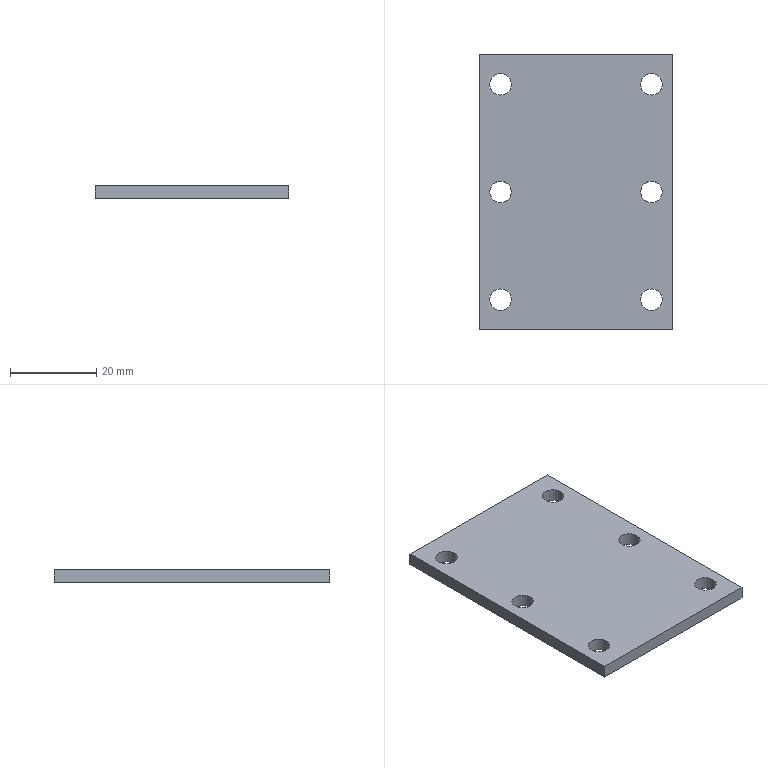Part | STEP file | 1-06.7 | 1 solid | 12 faces | box 45 x 64 x 3 mm | volume 8287 mm3 | plane 6 | cylinder 6 | commonest cylinder face diameters 5 x6
STEP:
#1=CARTESIAN_POINT('',(0.,0.,0.));
#2=DIRECTION('',(0.,0.,1.));
#3=DIRECTION('',(1.,0.,0.));
#4=AXIS2_PLACEMENT_3D('',#1,#2,#3);
#5=CARTESIAN_POINT('',(22.5,-32.,0.));
#6=VERTEX_POINT('',#5);
#7=CARTESIAN_POINT('',(22.5,32.,0.));
#8=VERTEX_POINT('',#7);
#9=CARTESIAN_POINT('',(22.5,-32.,0.));
#10=DIRECTION('',(0.,1.,0.));
#11=VECTOR('',#10,1.);
#12=LINE('',#9,#11);
#13=CARTESIAN_POINT('',(-9.5,0.,0.));
#14=DIRECTION('',(0.,0.,1.));
#15=DIRECTION('',(0.,1.,0.));
#16=AXIS2_PLACEMENT_3D('',#13,#14,#15);
#17=PLANE('',#16);
#18=CARTESIAN_POINT('',(-32.,-32.));
#19=DIRECTION('',(1.,0.));
#20=VECTOR('',#19,1.);
#21=LINE('',#18,#20);
#22=(GEOMETRIC_REPRESENTATION_CONTEXT(2)PARAMETRIC_REPRESENTATION_CONTEXT()REPRESENTATION_CONTEXT('',''));
#23=DEFINITIONAL_REPRESENTATION('',(#21),#22);
#24=PCURVE('',#17,#23);
#25=CARTESIAN_POINT('',(22.5,0.,-1.5));
#26=DIRECTION('',(-1.,0.,0.));
#27=DIRECTION('',(0.,1.,0.));
#28=AXIS2_PLACEMENT_3D('',#25,#26,#27);
#29=PLANE('',#28);
#30=CARTESIAN_POINT('',(-32.,-1.5));
#31=DIRECTION('',(1.,0.));
#32=VECTOR('',#31,1.);
#33=LINE('',#30,#32);
#34=(GEOMETRIC_REPRESENTATION_CONTEXT(2)PARAMETRIC_REPRESENTATION_CONTEXT()REPRESENTATION_CONTEXT('',''));
#35=DEFINITIONAL_REPRESENTATION('',(#33),#34);
#36=PCURVE('',#29,#35);
#37=SURFACE_CURVE('',#12,(#24,#36),.PCURVE_S1.);
#38=EDGE_CURVE('',#6,#8,#37,.T.);
#39=ORIENTED_EDGE('',*,*,#38,.T.);
#40=CARTESIAN_POINT('',(-22.5,32.,0.));
#41=VERTEX_POINT('',#40);
#42=CARTESIAN_POINT('',(22.5,32.,0.));
#43=DIRECTION('',(-1.,0.,0.));
#44=VECTOR('',#43,1.);
#45=LINE('',#42,#44);
#46=CARTESIAN_POINT('',(32.,-32.));
#47=DIRECTION('',(0.,1.));
#48=VECTOR('',#47,1.);
#49=LINE('',#46,#48);
#50=(GEOMETRIC_REPRESENTATION_CONTEXT(2)PARAMETRIC_REPRESENTATION_CONTEXT()REPRESENTATION_CONTEXT('',''));
#51=DEFINITIONAL_REPRESENTATION('',(#49),#50);
#52=PCURVE('',#17,#51);
#53=CARTESIAN_POINT('',(0.,32.,-1.5));
#54=DIRECTION('',(0.,-1.,0.));
#55=DIRECTION('',(-1.,0.,0.));
#56=AXIS2_PLACEMENT_3D('',#53,#54,#55);
#57=PLANE('',#56);
#58=CARTESIAN_POINT('',(-22.5,-1.5));
#59=DIRECTION('',(1.,0.));
#60=VECTOR('',#59,1.);
#61=LINE('',#58,#60);
#62=(GEOMETRIC_REPRESENTATION_CONTEXT(2)PARAMETRIC_REPRESENTATION_CONTEXT()REPRESENTATION_CONTEXT('',''));
#63=DEFINITIONAL_REPRESENTATION('',(#61),#62);
#64=PCURVE('',#57,#63);
#65=SURFACE_CURVE('',#45,(#52,#64),.PCURVE_S1.);
#66=EDGE_CURVE('',#8,#41,#65,.T.);
#67=ORIENTED_EDGE('',*,*,#66,.T.);
#68=CARTESIAN_POINT('',(-22.5,-32.,0.));
#69=VERTEX_POINT('',#68);
#70=CARTESIAN_POINT('',(-22.5,32.,0.));
#71=DIRECTION('',(0.,-1.,0.));
#72=VECTOR('',#71,1.);
#73=LINE('',#70,#72);
#74=CARTESIAN_POINT('',(32.,13.));
#75=DIRECTION('',(-1.,0.));
#76=VECTOR('',#75,1.);
#77=LINE('',#74,#76);
#78=(GEOMETRIC_REPRESENTATION_CONTEXT(2)PARAMETRIC_REPRESENTATION_CONTEXT()REPRESENTATION_CONTEXT('',''));
#79=DEFINITIONAL_REPRESENTATION('',(#77),#78);
#80=PCURVE('',#17,#79);
#81=CARTESIAN_POINT('',(-22.5,0.,-1.5));
#82=DIRECTION('',(1.,0.,0.));
#83=DIRECTION('',(0.,-1.,0.));
#84=AXIS2_PLACEMENT_3D('',#81,#82,#83);
#85=PLANE('',#84);
#86=CARTESIAN_POINT('',(-32.,-1.5));
#87=DIRECTION('',(1.,0.));
#88=VECTOR('',#87,1.);
#89=LINE('',#86,#88);
#90=(GEOMETRIC_REPRESENTATION_CONTEXT(2)PARAMETRIC_REPRESENTATION_CONTEXT()REPRESENTATION_CONTEXT('',''));
#91=DEFINITIONAL_REPRESENTATION('',(#89),#90);
#92=PCURVE('',#85,#91);
#93=SURFACE_CURVE('',#73,(#80,#92),.PCURVE_S1.);
#94=EDGE_CURVE('',#41,#69,#93,.T.);
#95=ORIENTED_EDGE('',*,*,#94,.T.);
#96=CARTESIAN_POINT('',(-22.5,-32.,0.));
#97=DIRECTION('',(1.,0.,0.));
#98=VECTOR('',#97,1.);
#99=LINE('',#96,#98);
#100=CARTESIAN_POINT('',(-32.,13.));
#101=DIRECTION('',(0.,-1.));
#102=VECTOR('',#101,1.);
#103=LINE('',#100,#102);
#104=(GEOMETRIC_REPRESENTATION_CONTEXT(2)PARAMETRIC_REPRESENTATION_CONTEXT()REPRESENTATION_CONTEXT('',''));
#105=DEFINITIONAL_REPRESENTATION('',(#103),#104);
#106=PCURVE('',#17,#105);
#107=CARTESIAN_POINT('',(0.,-32.,-1.5));
#108=DIRECTION('',(0.,1.,0.));
#109=DIRECTION('',(1.,0.,0.));
#110=AXIS2_PLACEMENT_3D('',#107,#108,#109);
#111=PLANE('',#110);
#112=CARTESIAN_POINT('',(-22.5,-1.5));
#113=DIRECTION('',(1.,0.));
#114=VECTOR('',#113,1.);
#115=LINE('',#112,#114);
#116=(GEOMETRIC_REPRESENTATION_CONTEXT(2)PARAMETRIC_REPRESENTATION_CONTEXT()REPRESENTATION_CONTEXT('',''));
#117=DEFINITIONAL_REPRESENTATION('',(#115),#116);
#118=PCURVE('',#111,#117);
#119=SURFACE_CURVE('',#99,(#106,#118),.PCURVE_S1.);
#120=EDGE_CURVE('',#69,#6,#119,.T.);
#121=ORIENTED_EDGE('',*,*,#120,.T.);
#122=EDGE_LOOP('',(#39,#67,#95,#121));
#123=FACE_BOUND('',#122,.T.);
#124=CARTESIAN_POINT('',(-17.5,-22.5,0.));
#125=VERTEX_POINT('',#124);
#126=CARTESIAN_POINT('',(-17.5,-25.,0.));
#127=DIRECTION('',(0.,0.,-1.));
#128=DIRECTION('',(0.,1.,0.));
#129=AXIS2_PLACEMENT_3D('',#126,#127,#128);
#130=CIRCLE('',#129,2.5);
#131=CARTESIAN_POINT('',(-22.5,8.));
#132=CARTESIAN_POINT('',(-22.5,3.67));
#133=CARTESIAN_POINT('',(-26.25,5.835));
#134=CARTESIAN_POINT('',(-30.,8.));
#135=CARTESIAN_POINT('',(-26.25,10.165));
#136=CARTESIAN_POINT('',(-22.5,12.33));
#137=CARTESIAN_POINT('',(-22.5,8.));
#138=(BOUNDED_CURVE()B_SPLINE_CURVE(2,(#131,#132,#133,#134,#135,#136,#137),.UNSPECIFIED.,.T.,.F.)B_SPLINE_CURVE_WITH_KNOTS((1,2,2,2,2,1),(-2.094,0.,2.094,4.189,6.283,8.378),.UNSPECIFIED.)CURVE()GEOMETRIC_REPRESENTATION_ITEM()RATIONAL_B_SPLINE_CURVE((1.,0.5,1.,0.5,1.,0.5,1.))REPRESENTATION_ITEM(''));
#139=(GEOMETRIC_REPRESENTATION_CONTEXT(2)PARAMETRIC_REPRESENTATION_CONTEXT()REPRESENTATION_CONTEXT('',''));
#140=DEFINITIONAL_REPRESENTATION('',(#138),#139);
#141=PCURVE('',#17,#140);
#142=CARTESIAN_POINT('',(-17.5,-25.,0.));
#143=DIRECTION('',(0.,0.,-1.));
#144=DIRECTION('',(0.,1.,0.));
#145=AXIS2_PLACEMENT_3D('',#142,#143,#144);
#146=CYLINDRICAL_SURFACE('',#145,2.5);
#147=CARTESIAN_POINT('',(0.,0.));
#148=DIRECTION('',(1.,0.));
#149=VECTOR('',#148,1.);
#150=LINE('',#147,#149);
#151=(GEOMETRIC_REPRESENTATION_CONTEXT(2)PARAMETRIC_REPRESENTATION_CONTEXT()REPRESENTATION_CONTEXT('',''));
#152=DEFINITIONAL_REPRESENTATION('',(#150),#151);
#153=PCURVE('',#146,#152);
#154=SURFACE_CURVE('',#130,(#141,#153),.PCURVE_S1.);
#155=EDGE_CURVE('',#125,#125,#154,.T.);
#156=ORIENTED_EDGE('',*,*,#155,.T.);
#157=EDGE_LOOP('',(#156));
#158=FACE_BOUND('',#157,.T.);
#159=CARTESIAN_POINT('',(-17.5,2.5,0.));
#160=VERTEX_POINT('',#159);
#161=CARTESIAN_POINT('',(-17.5,0.,0.));
#162=DIRECTION('',(0.,0.,-1.));
#163=DIRECTION('',(0.,1.,0.));
#164=AXIS2_PLACEMENT_3D('',#161,#162,#163);
#165=CIRCLE('',#164,2.5);
#166=CARTESIAN_POINT('',(2.5,8.));
#167=CARTESIAN_POINT('',(2.5,3.67));
#168=CARTESIAN_POINT('',(-1.25,5.835));
#169=CARTESIAN_POINT('',(-5.,8.));
#170=CARTESIAN_POINT('',(-1.25,10.165));
#171=CARTESIAN_POINT('',(2.5,12.33));
#172=CARTESIAN_POINT('',(2.5,8.));
#173=(BOUNDED_CURVE()B_SPLINE_CURVE(2,(#166,#167,#168,#169,#170,#171,#172),.UNSPECIFIED.,.T.,.F.)B_SPLINE_CURVE_WITH_KNOTS((1,2,2,2,2,1),(-2.094,0.,2.094,4.189,6.283,8.378),.UNSPECIFIED.)CURVE()GEOMETRIC_REPRESENTATION_ITEM()RATIONAL_B_SPLINE_CURVE((1.,0.5,1.,0.5,1.,0.5,1.))REPRESENTATION_ITEM(''));
#174=(GEOMETRIC_REPRESENTATION_CONTEXT(2)PARAMETRIC_REPRESENTATION_CONTEXT()REPRESENTATION_CONTEXT('',''));
#175=DEFINITIONAL_REPRESENTATION('',(#173),#174);
#176=PCURVE('',#17,#175);
#177=CARTESIAN_POINT('',(-17.5,0.,0.));
#178=DIRECTION('',(0.,0.,-1.));
#179=DIRECTION('',(0.,1.,0.));
#180=AXIS2_PLACEMENT_3D('',#177,#178,#179);
#181=CYLINDRICAL_SURFACE('',#180,2.5);
#182=CARTESIAN_POINT('',(0.,0.));
#183=DIRECTION('',(1.,0.));
#184=VECTOR('',#183,1.);
#185=LINE('',#182,#184);
#186=(GEOMETRIC_REPRESENTATION_CONTEXT(2)PARAMETRIC_REPRESENTATION_CONTEXT()REPRESENTATION_CONTEXT('',''));
#187=DEFINITIONAL_REPRESENTATION('',(#185),#186);
#188=PCURVE('',#181,#187);
#189=SURFACE_CURVE('',#165,(#176,#188),.PCURVE_S1.);
#190=EDGE_CURVE('',#160,#160,#189,.T.);
#191=ORIENTED_EDGE('',*,*,#190,.T.);
#192=EDGE_LOOP('',(#191));
#193=FACE_BOUND('',#192,.T.);
#194=CARTESIAN_POINT('',(-17.5,27.5,0.));
#195=VERTEX_POINT('',#194);
#196=CARTESIAN_POINT('',(-17.5,25.,0.));
#197=DIRECTION('',(0.,0.,-1.));
#198=DIRECTION('',(0.,1.,0.));
#199=AXIS2_PLACEMENT_3D('',#196,#197,#198);
#200=CIRCLE('',#199,2.5);
#201=CARTESIAN_POINT('',(27.5,8.));
#202=CARTESIAN_POINT('',(27.5,3.67));
#203=CARTESIAN_POINT('',(23.75,5.835));
#204=CARTESIAN_POINT('',(20.,8.));
#205=CARTESIAN_POINT('',(23.75,10.165));
#206=CARTESIAN_POINT('',(27.5,12.33));
#207=CARTESIAN_POINT('',(27.5,8.));
#208=(BOUNDED_CURVE()B_SPLINE_CURVE(2,(#201,#202,#203,#204,#205,#206,#207),.UNSPECIFIED.,.T.,.F.)B_SPLINE_CURVE_WITH_KNOTS((1,2,2,2,2,1),(-2.094,0.,2.094,4.189,6.283,8.378),.UNSPECIFIED.)CURVE()GEOMETRIC_REPRESENTATION_ITEM()RATIONAL_B_SPLINE_CURVE((1.,0.5,1.,0.5,1.,0.5,1.))REPRESENTATION_ITEM(''));
#209=(GEOMETRIC_REPRESENTATION_CONTEXT(2)PARAMETRIC_REPRESENTATION_CONTEXT()REPRESENTATION_CONTEXT('',''));
#210=DEFINITIONAL_REPRESENTATION('',(#208),#209);
#211=PCURVE('',#17,#210);
#212=CARTESIAN_POINT('',(-17.5,25.,0.));
#213=DIRECTION('',(0.,0.,-1.));
#214=DIRECTION('',(0.,1.,0.));
#215=AXIS2_PLACEMENT_3D('',#212,#213,#214);
#216=CYLINDRICAL_SURFACE('',#215,2.5);
#217=CARTESIAN_POINT('',(0.,0.));
#218=DIRECTION('',(1.,0.));
#219=VECTOR('',#218,1.);
#220=LINE('',#217,#219);
#221=(GEOMETRIC_REPRESENTATION_CONTEXT(2)PARAMETRIC_REPRESENTATION_CONTEXT()REPRESENTATION_CONTEXT('',''));
#222=DEFINITIONAL_REPRESENTATION('',(#220),#221);
#223=PCURVE('',#216,#222);
#224=SURFACE_CURVE('',#200,(#211,#223),.PCURVE_S1.);
#225=EDGE_CURVE('',#195,#195,#224,.T.);
#226=ORIENTED_EDGE('',*,*,#225,.T.);
#227=EDGE_LOOP('',(#226));
#228=FACE_BOUND('',#227,.T.);
#229=CARTESIAN_POINT('',(17.5,-22.5,0.));
#230=VERTEX_POINT('',#229);
#231=CARTESIAN_POINT('',(17.5,-25.,0.));
#232=DIRECTION('',(0.,0.,-1.));
#233=DIRECTION('',(0.,1.,0.));
#234=AXIS2_PLACEMENT_3D('',#231,#232,#233);
#235=CIRCLE('',#234,2.5);
#236=CARTESIAN_POINT('',(-22.5,-27.));
#237=CARTESIAN_POINT('',(-22.5,-31.33));
#238=CARTESIAN_POINT('',(-26.25,-29.165));
#239=CARTESIAN_POINT('',(-30.,-27.));
#240=CARTESIAN_POINT('',(-26.25,-24.835));
#241=CARTESIAN_POINT('',(-22.5,-22.67));
#242=CARTESIAN_POINT('',(-22.5,-27.));
#243=(BOUNDED_CURVE()B_SPLINE_CURVE(2,(#236,#237,#238,#239,#240,#241,#242),.UNSPECIFIED.,.T.,.F.)B_SPLINE_CURVE_WITH_KNOTS((1,2,2,2,2,1),(-2.094,0.,2.094,4.189,6.283,8.378),.UNSPECIFIED.)CURVE()GEOMETRIC_REPRESENTATION_ITEM()RATIONAL_B_SPLINE_CURVE((1.,0.5,1.,0.5,1.,0.5,1.))REPRESENTATION_ITEM(''));
#244=(GEOMETRIC_REPRESENTATION_CONTEXT(2)PARAMETRIC_REPRESENTATION_CONTEXT()REPRESENTATION_CONTEXT('',''));
#245=DEFINITIONAL_REPRESENTATION('',(#243),#244);
#246=PCURVE('',#17,#245);
#247=CARTESIAN_POINT('',(17.5,-25.,0.));
#248=DIRECTION('',(0.,0.,-1.));
#249=DIRECTION('',(0.,1.,0.));
#250=AXIS2_PLACEMENT_3D('',#247,#248,#249);
#251=CYLINDRICAL_SURFACE('',#250,2.5);
#252=CARTESIAN_POINT('',(0.,0.));
#253=DIRECTION('',(1.,0.));
#254=VECTOR('',#253,1.);
#255=LINE('',#252,#254);
#256=(GEOMETRIC_REPRESENTATION_CONTEXT(2)PARAMETRIC_REPRESENTATION_CONTEXT()REPRESENTATION_CONTEXT('',''));
#257=DEFINITIONAL_REPRESENTATION('',(#255),#256);
#258=PCURVE('',#251,#257);
#259=SURFACE_CURVE('',#235,(#246,#258),.PCURVE_S1.);
#260=EDGE_CURVE('',#230,#230,#259,.T.);
#261=ORIENTED_EDGE('',*,*,#260,.T.);
#262=EDGE_LOOP('',(#261));
#263=FACE_BOUND('',#262,.T.);
#264=CARTESIAN_POINT('',(17.5,2.5,0.));
#265=VERTEX_POINT('',#264);
#266=CARTESIAN_POINT('',(17.5,0.,0.));
#267=DIRECTION('',(0.,0.,-1.));
#268=DIRECTION('',(0.,1.,0.));
#269=AXIS2_PLACEMENT_3D('',#266,#267,#268);
#270=CIRCLE('',#269,2.5);
#271=CARTESIAN_POINT('',(2.5,-27.));
#272=CARTESIAN_POINT('',(2.5,-31.33));
#273=CARTESIAN_POINT('',(-1.25,-29.165));
#274=CARTESIAN_POINT('',(-5.,-27.));
#275=CARTESIAN_POINT('',(-1.25,-24.835));
#276=CARTESIAN_POINT('',(2.5,-22.67));
#277=CARTESIAN_POINT('',(2.5,-27.));
#278=(BOUNDED_CURVE()B_SPLINE_CURVE(2,(#271,#272,#273,#274,#275,#276,#277),.UNSPECIFIED.,.T.,.F.)B_SPLINE_CURVE_WITH_KNOTS((1,2,2,2,2,1),(-2.094,0.,2.094,4.189,6.283,8.378),.UNSPECIFIED.)CURVE()GEOMETRIC_REPRESENTATION_ITEM()RATIONAL_B_SPLINE_CURVE((1.,0.5,1.,0.5,1.,0.5,1.))REPRESENTATION_ITEM(''));
#279=(GEOMETRIC_REPRESENTATION_CONTEXT(2)PARAMETRIC_REPRESENTATION_CONTEXT()REPRESENTATION_CONTEXT('',''));
#280=DEFINITIONAL_REPRESENTATION('',(#278),#279);
#281=PCURVE('',#17,#280);
#282=CARTESIAN_POINT('',(17.5,0.,0.));
#283=DIRECTION('',(0.,0.,-1.));
#284=DIRECTION('',(0.,1.,0.));
#285=AXIS2_PLACEMENT_3D('',#282,#283,#284);
#286=CYLINDRICAL_SURFACE('',#285,2.5);
#287=CARTESIAN_POINT('',(0.,0.));
#288=DIRECTION('',(1.,0.));
#289=VECTOR('',#288,1.);
#290=LINE('',#287,#289);
#291=(GEOMETRIC_REPRESENTATION_CONTEXT(2)PARAMETRIC_REPRESENTATION_CONTEXT()REPRESENTATION_CONTEXT('',''));
#292=DEFINITIONAL_REPRESENTATION('',(#290),#291);
#293=PCURVE('',#286,#292);
#294=SURFACE_CURVE('',#270,(#281,#293),.PCURVE_S1.);
#295=EDGE_CURVE('',#265,#265,#294,.T.);
#296=ORIENTED_EDGE('',*,*,#295,.T.);
#297=EDGE_LOOP('',(#296));
#298=FACE_BOUND('',#297,.T.);
#299=CARTESIAN_POINT('',(17.5,27.5,0.));
#300=VERTEX_POINT('',#299);
#301=CARTESIAN_POINT('',(17.5,25.,0.));
#302=DIRECTION('',(0.,0.,-1.));
#303=DIRECTION('',(0.,1.,0.));
#304=AXIS2_PLACEMENT_3D('',#301,#302,#303);
#305=CIRCLE('',#304,2.5);
#306=CARTESIAN_POINT('',(27.5,-27.));
#307=CARTESIAN_POINT('',(27.5,-31.33));
#308=CARTESIAN_POINT('',(23.75,-29.165));
#309=CARTESIAN_POINT('',(20.,-27.));
#310=CARTESIAN_POINT('',(23.75,-24.835));
#311=CARTESIAN_POINT('',(27.5,-22.67));
#312=CARTESIAN_POINT('',(27.5,-27.));
#313=(BOUNDED_CURVE()B_SPLINE_CURVE(2,(#306,#307,#308,#309,#310,#311,#312),.UNSPECIFIED.,.T.,.F.)B_SPLINE_CURVE_WITH_KNOTS((1,2,2,2,2,1),(-2.094,0.,2.094,4.189,6.283,8.378),.UNSPECIFIED.)CURVE()GEOMETRIC_REPRESENTATION_ITEM()RATIONAL_B_SPLINE_CURVE((1.,0.5,1.,0.5,1.,0.5,1.))REPRESENTATION_ITEM(''));
#314=(GEOMETRIC_REPRESENTATION_CONTEXT(2)PARAMETRIC_REPRESENTATION_CONTEXT()REPRESENTATION_CONTEXT('',''));
#315=DEFINITIONAL_REPRESENTATION('',(#313),#314);
#316=PCURVE('',#17,#315);
#317=CARTESIAN_POINT('',(17.5,25.,0.));
#318=DIRECTION('',(0.,0.,-1.));
#319=DIRECTION('',(0.,1.,0.));
#320=AXIS2_PLACEMENT_3D('',#317,#318,#319);
#321=CYLINDRICAL_SURFACE('',#320,2.5);
#322=CARTESIAN_POINT('',(0.,0.));
#323=DIRECTION('',(1.,0.));
#324=VECTOR('',#323,1.);
#325=LINE('',#322,#324);
#326=(GEOMETRIC_REPRESENTATION_CONTEXT(2)PARAMETRIC_REPRESENTATION_CONTEXT()REPRESENTATION_CONTEXT('',''));
#327=DEFINITIONAL_REPRESENTATION('',(#325),#326);
#328=PCURVE('',#321,#327);
#329=SURFACE_CURVE('',#305,(#316,#328),.PCURVE_S1.);
#330=EDGE_CURVE('',#300,#300,#329,.T.);
#331=ORIENTED_EDGE('',*,*,#330,.T.);
#332=EDGE_LOOP('',(#331));
#333=FACE_BOUND('',#332,.T.);
#334=ADVANCED_FACE('',(#123,#158,#193,#228,#263,#298,#333),#17,.T.);
#335=CARTESIAN_POINT('',(22.5,-32.,-3.));
#336=VERTEX_POINT('',#335);
#337=CARTESIAN_POINT('',(22.5,32.,-3.));
#338=VERTEX_POINT('',#337);
#339=CARTESIAN_POINT('',(22.5,-32.,-3.));
#340=DIRECTION('',(0.,1.,0.));
#341=VECTOR('',#340,1.);
#342=LINE('',#339,#341);
#343=CARTESIAN_POINT('',(-9.5,0.,-3.));
#344=DIRECTION('',(0.,0.,1.));
#345=DIRECTION('',(0.,1.,0.));
#346=AXIS2_PLACEMENT_3D('',#343,#344,#345);
#347=PLANE('',#346);
#348=CARTESIAN_POINT('',(-32.,-32.));
#349=DIRECTION('',(1.,0.));
#350=VECTOR('',#349,1.);
#351=LINE('',#348,#350);
#352=(GEOMETRIC_REPRESENTATION_CONTEXT(2)PARAMETRIC_REPRESENTATION_CONTEXT()REPRESENTATION_CONTEXT('',''));
#353=DEFINITIONAL_REPRESENTATION('',(#351),#352);
#354=PCURVE('',#347,#353);
#355=CARTESIAN_POINT('',(-32.,1.5));
#356=DIRECTION('',(1.,0.));
#357=VECTOR('',#356,1.);
#358=LINE('',#355,#357);
#359=(GEOMETRIC_REPRESENTATION_CONTEXT(2)PARAMETRIC_REPRESENTATION_CONTEXT()REPRESENTATION_CONTEXT('',''));
#360=DEFINITIONAL_REPRESENTATION('',(#358),#359);
#361=PCURVE('',#29,#360);
#362=SURFACE_CURVE('',#342,(#354,#361),.PCURVE_S1.);
#363=EDGE_CURVE('',#336,#338,#362,.T.);
#364=ORIENTED_EDGE('',*,*,#363,.T.);
#365=CARTESIAN_POINT('',(-22.5,32.,-3.));
#366=VERTEX_POINT('',#365);
#367=CARTESIAN_POINT('',(22.5,32.,-3.));
#368=DIRECTION('',(-1.,0.,0.));
#369=VECTOR('',#368,1.);
#370=LINE('',#367,#369);
#371=CARTESIAN_POINT('',(32.,-32.));
#372=DIRECTION('',(0.,1.));
#373=VECTOR('',#372,1.);
#374=LINE('',#371,#373);
#375=(GEOMETRIC_REPRESENTATION_CONTEXT(2)PARAMETRIC_REPRESENTATION_CONTEXT()REPRESENTATION_CONTEXT('',''));
#376=DEFINITIONAL_REPRESENTATION('',(#374),#375);
#377=PCURVE('',#347,#376);
#378=CARTESIAN_POINT('',(-22.5,1.5));
#379=DIRECTION('',(1.,0.));
#380=VECTOR('',#379,1.);
#381=LINE('',#378,#380);
#382=(GEOMETRIC_REPRESENTATION_CONTEXT(2)PARAMETRIC_REPRESENTATION_CONTEXT()REPRESENTATION_CONTEXT('',''));
#383=DEFINITIONAL_REPRESENTATION('',(#381),#382);
#384=PCURVE('',#57,#383);
#385=SURFACE_CURVE('',#370,(#377,#384),.PCURVE_S1.);
#386=EDGE_CURVE('',#338,#366,#385,.T.);
#387=ORIENTED_EDGE('',*,*,#386,.T.);
#388=CARTESIAN_POINT('',(-22.5,-32.,-3.));
#389=VERTEX_POINT('',#388);
#390=CARTESIAN_POINT('',(-22.5,32.,-3.));
#391=DIRECTION('',(0.,-1.,0.));
#392=VECTOR('',#391,1.);
#393=LINE('',#390,#392);
#394=CARTESIAN_POINT('',(32.,13.));
#395=DIRECTION('',(-1.,0.));
#396=VECTOR('',#395,1.);
#397=LINE('',#394,#396);
#398=(GEOMETRIC_REPRESENTATION_CONTEXT(2)PARAMETRIC_REPRESENTATION_CONTEXT()REPRESENTATION_CONTEXT('',''));
#399=DEFINITIONAL_REPRESENTATION('',(#397),#398);
#400=PCURVE('',#347,#399);
#401=CARTESIAN_POINT('',(-32.,1.5));
#402=DIRECTION('',(1.,0.));
#403=VECTOR('',#402,1.);
#404=LINE('',#401,#403);
#405=(GEOMETRIC_REPRESENTATION_CONTEXT(2)PARAMETRIC_REPRESENTATION_CONTEXT()REPRESENTATION_CONTEXT('',''));
#406=DEFINITIONAL_REPRESENTATION('',(#404),#405);
#407=PCURVE('',#85,#406);
#408=SURFACE_CURVE('',#393,(#400,#407),.PCURVE_S1.);
#409=EDGE_CURVE('',#366,#389,#408,.T.);
#410=ORIENTED_EDGE('',*,*,#409,.T.);
#411=CARTESIAN_POINT('',(-22.5,-32.,-3.));
#412=DIRECTION('',(1.,0.,0.));
#413=VECTOR('',#412,1.);
#414=LINE('',#411,#413);
#415=CARTESIAN_POINT('',(-32.,13.));
#416=DIRECTION('',(0.,-1.));
#417=VECTOR('',#416,1.);
#418=LINE('',#415,#417);
#419=(GEOMETRIC_REPRESENTATION_CONTEXT(2)PARAMETRIC_REPRESENTATION_CONTEXT()REPRESENTATION_CONTEXT('',''));
#420=DEFINITIONAL_REPRESENTATION('',(#418),#419);
#421=PCURVE('',#347,#420);
#422=CARTESIAN_POINT('',(-22.5,1.5));
#423=DIRECTION('',(1.,0.));
#424=VECTOR('',#423,1.);
#425=LINE('',#422,#424);
#426=(GEOMETRIC_REPRESENTATION_CONTEXT(2)PARAMETRIC_REPRESENTATION_CONTEXT()REPRESENTATION_CONTEXT('',''));
#427=DEFINITIONAL_REPRESENTATION('',(#425),#426);
#428=PCURVE('',#111,#427);
#429=SURFACE_CURVE('',#414,(#421,#428),.PCURVE_S1.);
#430=EDGE_CURVE('',#389,#336,#429,.T.);
#431=ORIENTED_EDGE('',*,*,#430,.T.);
#432=EDGE_LOOP('',(#364,#387,#410,#431));
#433=FACE_BOUND('',#432,.F.);
#434=CARTESIAN_POINT('',(-17.5,-22.5,-3.));
#435=VERTEX_POINT('',#434);
#436=CARTESIAN_POINT('',(-17.5,-25.,-3.));
#437=DIRECTION('',(0.,0.,-1.));
#438=DIRECTION('',(0.,1.,0.));
#439=AXIS2_PLACEMENT_3D('',#436,#437,#438);
#440=CIRCLE('',#439,2.5);
#441=CARTESIAN_POINT('',(-22.5,8.));
#442=CARTESIAN_POINT('',(-22.5,3.67));
#443=CARTESIAN_POINT('',(-26.25,5.835));
#444=CARTESIAN_POINT('',(-30.,8.));
#445=CARTESIAN_POINT('',(-26.25,10.165));
#446=CARTESIAN_POINT('',(-22.5,12.33));
#447=CARTESIAN_POINT('',(-22.5,8.));
#448=(BOUNDED_CURVE()B_SPLINE_CURVE(2,(#441,#442,#443,#444,#445,#446,#447),.UNSPECIFIED.,.T.,.F.)B_SPLINE_CURVE_WITH_KNOTS((1,2,2,2,2,1),(-2.094,0.,2.094,4.189,6.283,8.378),.UNSPECIFIED.)CURVE()GEOMETRIC_REPRESENTATION_ITEM()RATIONAL_B_SPLINE_CURVE((1.,0.5,1.,0.5,1.,0.5,1.))REPRESENTATION_ITEM(''));
#449=(GEOMETRIC_REPRESENTATION_CONTEXT(2)PARAMETRIC_REPRESENTATION_CONTEXT()REPRESENTATION_CONTEXT('',''));
#450=DEFINITIONAL_REPRESENTATION('',(#448),#449);
#451=PCURVE('',#347,#450);
#452=CARTESIAN_POINT('',(0.,3.));
#453=DIRECTION('',(1.,0.));
#454=VECTOR('',#453,1.);
#455=LINE('',#452,#454);
#456=(GEOMETRIC_REPRESENTATION_CONTEXT(2)PARAMETRIC_REPRESENTATION_CONTEXT()REPRESENTATION_CONTEXT('',''));
#457=DEFINITIONAL_REPRESENTATION('',(#455),#456);
#458=PCURVE('',#146,#457);
#459=SURFACE_CURVE('',#440,(#451,#458),.PCURVE_S1.);
#460=EDGE_CURVE('',#435,#435,#459,.T.);
#461=ORIENTED_EDGE('',*,*,#460,.T.);
#462=EDGE_LOOP('',(#461));
#463=FACE_BOUND('',#462,.F.);
#464=CARTESIAN_POINT('',(-17.5,2.5,-3.));
#465=VERTEX_POINT('',#464);
#466=CARTESIAN_POINT('',(-17.5,0.,-3.));
#467=DIRECTION('',(0.,0.,-1.));
#468=DIRECTION('',(0.,1.,0.));
#469=AXIS2_PLACEMENT_3D('',#466,#467,#468);
#470=CIRCLE('',#469,2.5);
#471=CARTESIAN_POINT('',(2.5,8.));
#472=CARTESIAN_POINT('',(2.5,3.67));
#473=CARTESIAN_POINT('',(-1.25,5.835));
#474=CARTESIAN_POINT('',(-5.,8.));
#475=CARTESIAN_POINT('',(-1.25,10.165));
#476=CARTESIAN_POINT('',(2.5,12.33));
#477=CARTESIAN_POINT('',(2.5,8.));
#478=(BOUNDED_CURVE()B_SPLINE_CURVE(2,(#471,#472,#473,#474,#475,#476,#477),.UNSPECIFIED.,.T.,.F.)B_SPLINE_CURVE_WITH_KNOTS((1,2,2,2,2,1),(-2.094,0.,2.094,4.189,6.283,8.378),.UNSPECIFIED.)CURVE()GEOMETRIC_REPRESENTATION_ITEM()RATIONAL_B_SPLINE_CURVE((1.,0.5,1.,0.5,1.,0.5,1.))REPRESENTATION_ITEM(''));
#479=(GEOMETRIC_REPRESENTATION_CONTEXT(2)PARAMETRIC_REPRESENTATION_CONTEXT()REPRESENTATION_CONTEXT('',''));
#480=DEFINITIONAL_REPRESENTATION('',(#478),#479);
#481=PCURVE('',#347,#480);
#482=CARTESIAN_POINT('',(0.,3.));
#483=DIRECTION('',(1.,0.));
#484=VECTOR('',#483,1.);
#485=LINE('',#482,#484);
#486=(GEOMETRIC_REPRESENTATION_CONTEXT(2)PARAMETRIC_REPRESENTATION_CONTEXT()REPRESENTATION_CONTEXT('',''));
#487=DEFINITIONAL_REPRESENTATION('',(#485),#486);
#488=PCURVE('',#181,#487);
#489=SURFACE_CURVE('',#470,(#481,#488),.PCURVE_S1.);
#490=EDGE_CURVE('',#465,#465,#489,.T.);
#491=ORIENTED_EDGE('',*,*,#490,.T.);
#492=EDGE_LOOP('',(#491));
#493=FACE_BOUND('',#492,.F.);
#494=CARTESIAN_POINT('',(-17.5,27.5,-3.));
#495=VERTEX_POINT('',#494);
#496=CARTESIAN_POINT('',(-17.5,25.,-3.));
#497=DIRECTION('',(0.,0.,-1.));
#498=DIRECTION('',(0.,1.,0.));
#499=AXIS2_PLACEMENT_3D('',#496,#497,#498);
#500=CIRCLE('',#499,2.5);
#501=CARTESIAN_POINT('',(27.5,8.));
#502=CARTESIAN_POINT('',(27.5,3.67));
#503=CARTESIAN_POINT('',(23.75,5.835));
#504=CARTESIAN_POINT('',(20.,8.));
#505=CARTESIAN_POINT('',(23.75,10.165));
#506=CARTESIAN_POINT('',(27.5,12.33));
#507=CARTESIAN_POINT('',(27.5,8.));
#508=(BOUNDED_CURVE()B_SPLINE_CURVE(2,(#501,#502,#503,#504,#505,#506,#507),.UNSPECIFIED.,.T.,.F.)B_SPLINE_CURVE_WITH_KNOTS((1,2,2,2,2,1),(-2.094,0.,2.094,4.189,6.283,8.378),.UNSPECIFIED.)CURVE()GEOMETRIC_REPRESENTATION_ITEM()RATIONAL_B_SPLINE_CURVE((1.,0.5,1.,0.5,1.,0.5,1.))REPRESENTATION_ITEM(''));
#509=(GEOMETRIC_REPRESENTATION_CONTEXT(2)PARAMETRIC_REPRESENTATION_CONTEXT()REPRESENTATION_CONTEXT('',''));
#510=DEFINITIONAL_REPRESENTATION('',(#508),#509);
#511=PCURVE('',#347,#510);
#512=CARTESIAN_POINT('',(0.,3.));
#513=DIRECTION('',(1.,0.));
#514=VECTOR('',#513,1.);
#515=LINE('',#512,#514);
#516=(GEOMETRIC_REPRESENTATION_CONTEXT(2)PARAMETRIC_REPRESENTATION_CONTEXT()REPRESENTATION_CONTEXT('',''));
#517=DEFINITIONAL_REPRESENTATION('',(#515),#516);
#518=PCURVE('',#216,#517);
#519=SURFACE_CURVE('',#500,(#511,#518),.PCURVE_S1.);
#520=EDGE_CURVE('',#495,#495,#519,.T.);
#521=ORIENTED_EDGE('',*,*,#520,.T.);
#522=EDGE_LOOP('',(#521));
#523=FACE_BOUND('',#522,.F.);
#524=CARTESIAN_POINT('',(17.5,-22.5,-3.));
#525=VERTEX_POINT('',#524);
#526=CARTESIAN_POINT('',(17.5,-25.,-3.));
#527=DIRECTION('',(0.,0.,-1.));
#528=DIRECTION('',(0.,1.,0.));
#529=AXIS2_PLACEMENT_3D('',#526,#527,#528);
#530=CIRCLE('',#529,2.5);
#531=CARTESIAN_POINT('',(-22.5,-27.));
#532=CARTESIAN_POINT('',(-22.5,-31.33));
#533=CARTESIAN_POINT('',(-26.25,-29.165));
#534=CARTESIAN_POINT('',(-30.,-27.));
#535=CARTESIAN_POINT('',(-26.25,-24.835));
#536=CARTESIAN_POINT('',(-22.5,-22.67));
#537=CARTESIAN_POINT('',(-22.5,-27.));
#538=(BOUNDED_CURVE()B_SPLINE_CURVE(2,(#531,#532,#533,#534,#535,#536,#537),.UNSPECIFIED.,.T.,.F.)B_SPLINE_CURVE_WITH_KNOTS((1,2,2,2,2,1),(-2.094,0.,2.094,4.189,6.283,8.378),.UNSPECIFIED.)CURVE()GEOMETRIC_REPRESENTATION_ITEM()RATIONAL_B_SPLINE_CURVE((1.,0.5,1.,0.5,1.,0.5,1.))REPRESENTATION_ITEM(''));
#539=(GEOMETRIC_REPRESENTATION_CONTEXT(2)PARAMETRIC_REPRESENTATION_CONTEXT()REPRESENTATION_CONTEXT('',''));
#540=DEFINITIONAL_REPRESENTATION('',(#538),#539);
#541=PCURVE('',#347,#540);
#542=CARTESIAN_POINT('',(0.,3.));
#543=DIRECTION('',(1.,0.));
#544=VECTOR('',#543,1.);
#545=LINE('',#542,#544);
#546=(GEOMETRIC_REPRESENTATION_CONTEXT(2)PARAMETRIC_REPRESENTATION_CONTEXT()REPRESENTATION_CONTEXT('',''));
#547=DEFINITIONAL_REPRESENTATION('',(#545),#546);
#548=PCURVE('',#251,#547);
#549=SURFACE_CURVE('',#530,(#541,#548),.PCURVE_S1.);
#550=EDGE_CURVE('',#525,#525,#549,.T.);
#551=ORIENTED_EDGE('',*,*,#550,.T.);
#552=EDGE_LOOP('',(#551));
#553=FACE_BOUND('',#552,.F.);
#554=CARTESIAN_POINT('',(17.5,2.5,-3.));
#555=VERTEX_POINT('',#554);
#556=CARTESIAN_POINT('',(17.5,0.,-3.));
#557=DIRECTION('',(0.,0.,-1.));
#558=DIRECTION('',(0.,1.,0.));
#559=AXIS2_PLACEMENT_3D('',#556,#557,#558);
#560=CIRCLE('',#559,2.5);
#561=CARTESIAN_POINT('',(2.5,-27.));
#562=CARTESIAN_POINT('',(2.5,-31.33));
#563=CARTESIAN_POINT('',(-1.25,-29.165));
#564=CARTESIAN_POINT('',(-5.,-27.));
#565=CARTESIAN_POINT('',(-1.25,-24.835));
#566=CARTESIAN_POINT('',(2.5,-22.67));
#567=CARTESIAN_POINT('',(2.5,-27.));
#568=(BOUNDED_CURVE()B_SPLINE_CURVE(2,(#561,#562,#563,#564,#565,#566,#567),.UNSPECIFIED.,.T.,.F.)B_SPLINE_CURVE_WITH_KNOTS((1,2,2,2,2,1),(-2.094,0.,2.094,4.189,6.283,8.378),.UNSPECIFIED.)CURVE()GEOMETRIC_REPRESENTATION_ITEM()RATIONAL_B_SPLINE_CURVE((1.,0.5,1.,0.5,1.,0.5,1.))REPRESENTATION_ITEM(''));
#569=(GEOMETRIC_REPRESENTATION_CONTEXT(2)PARAMETRIC_REPRESENTATION_CONTEXT()REPRESENTATION_CONTEXT('',''));
#570=DEFINITIONAL_REPRESENTATION('',(#568),#569);
#571=PCURVE('',#347,#570);
#572=CARTESIAN_POINT('',(0.,3.));
#573=DIRECTION('',(1.,0.));
#574=VECTOR('',#573,1.);
#575=LINE('',#572,#574);
#576=(GEOMETRIC_REPRESENTATION_CONTEXT(2)PARAMETRIC_REPRESENTATION_CONTEXT()REPRESENTATION_CONTEXT('',''));
#577=DEFINITIONAL_REPRESENTATION('',(#575),#576);
#578=PCURVE('',#286,#577);
#579=SURFACE_CURVE('',#560,(#571,#578),.PCURVE_S1.);
#580=EDGE_CURVE('',#555,#555,#579,.T.);
#581=ORIENTED_EDGE('',*,*,#580,.T.);
#582=EDGE_LOOP('',(#581));
#583=FACE_BOUND('',#582,.F.);
#584=CARTESIAN_POINT('',(17.5,27.5,-3.));
#585=VERTEX_POINT('',#584);
#586=CARTESIAN_POINT('',(17.5,25.,-3.));
#587=DIRECTION('',(0.,0.,-1.));
#588=DIRECTION('',(0.,1.,0.));
#589=AXIS2_PLACEMENT_3D('',#586,#587,#588);
#590=CIRCLE('',#589,2.5);
#591=CARTESIAN_POINT('',(27.5,-27.));
#592=CARTESIAN_POINT('',(27.5,-31.33));
#593=CARTESIAN_POINT('',(23.75,-29.165));
#594=CARTESIAN_POINT('',(20.,-27.));
#595=CARTESIAN_POINT('',(23.75,-24.835));
#596=CARTESIAN_POINT('',(27.5,-22.67));
#597=CARTESIAN_POINT('',(27.5,-27.));
#598=(BOUNDED_CURVE()B_SPLINE_CURVE(2,(#591,#592,#593,#594,#595,#596,#597),.UNSPECIFIED.,.T.,.F.)B_SPLINE_CURVE_WITH_KNOTS((1,2,2,2,2,1),(-2.094,0.,2.094,4.189,6.283,8.378),.UNSPECIFIED.)CURVE()GEOMETRIC_REPRESENTATION_ITEM()RATIONAL_B_SPLINE_CURVE((1.,0.5,1.,0.5,1.,0.5,1.))REPRESENTATION_ITEM(''));
#599=(GEOMETRIC_REPRESENTATION_CONTEXT(2)PARAMETRIC_REPRESENTATION_CONTEXT()REPRESENTATION_CONTEXT('',''));
#600=DEFINITIONAL_REPRESENTATION('',(#598),#599);
#601=PCURVE('',#347,#600);
#602=CARTESIAN_POINT('',(0.,3.));
#603=DIRECTION('',(1.,0.));
#604=VECTOR('',#603,1.);
#605=LINE('',#602,#604);
#606=(GEOMETRIC_REPRESENTATION_CONTEXT(2)PARAMETRIC_REPRESENTATION_CONTEXT()REPRESENTATION_CONTEXT('',''));
#607=DEFINITIONAL_REPRESENTATION('',(#605),#606);
#608=PCURVE('',#321,#607);
#609=SURFACE_CURVE('',#590,(#601,#608),.PCURVE_S1.);
#610=EDGE_CURVE('',#585,#585,#609,.T.);
#611=ORIENTED_EDGE('',*,*,#610,.T.);
#612=EDGE_LOOP('',(#611));
#613=FACE_BOUND('',#612,.F.);
#614=ADVANCED_FACE('',(#433,#463,#493,#523,#553,#583,#613),#347,.F.);
#615=ORIENTED_EDGE('',*,*,#38,.T.);
#616=CARTESIAN_POINT('',(22.5,32.,0.));
#617=DIRECTION('',(0.,0.,-1.));
#618=VECTOR('',#617,1.);
#619=LINE('',#616,#618);
#620=CARTESIAN_POINT('',(32.,-1.5));
#621=DIRECTION('',(0.,1.));
#622=VECTOR('',#621,1.);
#623=LINE('',#620,#622);
#624=(GEOMETRIC_REPRESENTATION_CONTEXT(2)PARAMETRIC_REPRESENTATION_CONTEXT()REPRESENTATION_CONTEXT('',''));
#625=DEFINITIONAL_REPRESENTATION('',(#623),#624);
#626=PCURVE('',#29,#625);
#627=CARTESIAN_POINT('',(-22.5,-1.5));
#628=DIRECTION('',(0.,1.));
#629=VECTOR('',#628,1.);
#630=LINE('',#627,#629);
#631=(GEOMETRIC_REPRESENTATION_CONTEXT(2)PARAMETRIC_REPRESENTATION_CONTEXT()REPRESENTATION_CONTEXT('',''));
#632=DEFINITIONAL_REPRESENTATION('',(#630),#631);
#633=PCURVE('',#57,#632);
#634=SURFACE_CURVE('',#619,(#626,#633),.PCURVE_S1.);
#635=EDGE_CURVE('',#8,#338,#634,.T.);
#636=ORIENTED_EDGE('',*,*,#635,.T.);
#637=ORIENTED_EDGE('',*,*,#363,.F.);
#638=CARTESIAN_POINT('',(22.5,-32.,0.));
#639=DIRECTION('',(0.,0.,-1.));
#640=VECTOR('',#639,1.);
#641=LINE('',#638,#640);
#642=CARTESIAN_POINT('',(-32.,-1.5));
#643=DIRECTION('',(0.,1.));
#644=VECTOR('',#643,1.);
#645=LINE('',#642,#644);
#646=(GEOMETRIC_REPRESENTATION_CONTEXT(2)PARAMETRIC_REPRESENTATION_CONTEXT()REPRESENTATION_CONTEXT('',''));
#647=DEFINITIONAL_REPRESENTATION('',(#645),#646);
#648=PCURVE('',#29,#647);
#649=CARTESIAN_POINT('',(22.5,-1.5));
#650=DIRECTION('',(0.,1.));
#651=VECTOR('',#650,1.);
#652=LINE('',#649,#651);
#653=(GEOMETRIC_REPRESENTATION_CONTEXT(2)PARAMETRIC_REPRESENTATION_CONTEXT()REPRESENTATION_CONTEXT('',''));
#654=DEFINITIONAL_REPRESENTATION('',(#652),#653);
#655=PCURVE('',#111,#654);
#656=SURFACE_CURVE('',#641,(#648,#655),.PCURVE_S1.);
#657=EDGE_CURVE('',#6,#336,#656,.T.);
#658=ORIENTED_EDGE('',*,*,#657,.F.);
#659=EDGE_LOOP('',(#615,#636,#637,#658));
#660=FACE_BOUND('',#659,.F.);
#661=ADVANCED_FACE('',(#660),#29,.F.);
#662=ORIENTED_EDGE('',*,*,#66,.T.);
#663=CARTESIAN_POINT('',(-22.5,32.,0.));
#664=DIRECTION('',(0.,0.,-1.));
#665=VECTOR('',#664,1.);
#666=LINE('',#663,#665);
#667=CARTESIAN_POINT('',(22.5,-1.5));
#668=DIRECTION('',(0.,1.));
#669=VECTOR('',#668,1.);
#670=LINE('',#667,#669);
#671=(GEOMETRIC_REPRESENTATION_CONTEXT(2)PARAMETRIC_REPRESENTATION_CONTEXT()REPRESENTATION_CONTEXT('',''));
#672=DEFINITIONAL_REPRESENTATION('',(#670),#671);
#673=PCURVE('',#57,#672);
#674=CARTESIAN_POINT('',(-32.,-1.5));
#675=DIRECTION('',(0.,1.));
#676=VECTOR('',#675,1.);
#677=LINE('',#674,#676);
#678=(GEOMETRIC_REPRESENTATION_CONTEXT(2)PARAMETRIC_REPRESENTATION_CONTEXT()REPRESENTATION_CONTEXT('',''));
#679=DEFINITIONAL_REPRESENTATION('',(#677),#678);
#680=PCURVE('',#85,#679);
#681=SURFACE_CURVE('',#666,(#673,#680),.PCURVE_S1.);
#682=EDGE_CURVE('',#41,#366,#681,.T.);
#683=ORIENTED_EDGE('',*,*,#682,.T.);
#684=ORIENTED_EDGE('',*,*,#386,.F.);
#685=ORIENTED_EDGE('',*,*,#635,.F.);
#686=EDGE_LOOP('',(#662,#683,#684,#685));
#687=FACE_BOUND('',#686,.F.);
#688=ADVANCED_FACE('',(#687),#57,.F.);
#689=ORIENTED_EDGE('',*,*,#94,.T.);
#690=CARTESIAN_POINT('',(-22.5,-32.,0.));
#691=DIRECTION('',(0.,0.,-1.));
#692=VECTOR('',#691,1.);
#693=LINE('',#690,#692);
#694=CARTESIAN_POINT('',(32.,-1.5));
#695=DIRECTION('',(0.,1.));
#696=VECTOR('',#695,1.);
#697=LINE('',#694,#696);
#698=(GEOMETRIC_REPRESENTATION_CONTEXT(2)PARAMETRIC_REPRESENTATION_CONTEXT()REPRESENTATION_CONTEXT('',''));
#699=DEFINITIONAL_REPRESENTATION('',(#697),#698);
#700=PCURVE('',#85,#699);
#701=CARTESIAN_POINT('',(-22.5,-1.5));
#702=DIRECTION('',(0.,1.));
#703=VECTOR('',#702,1.);
#704=LINE('',#701,#703);
#705=(GEOMETRIC_REPRESENTATION_CONTEXT(2)PARAMETRIC_REPRESENTATION_CONTEXT()REPRESENTATION_CONTEXT('',''));
#706=DEFINITIONAL_REPRESENTATION('',(#704),#705);
#707=PCURVE('',#111,#706);
#708=SURFACE_CURVE('',#693,(#700,#707),.PCURVE_S1.);
#709=EDGE_CURVE('',#69,#389,#708,.T.);
#710=ORIENTED_EDGE('',*,*,#709,.T.);
#711=ORIENTED_EDGE('',*,*,#409,.F.);
#712=ORIENTED_EDGE('',*,*,#682,.F.);
#713=EDGE_LOOP('',(#689,#710,#711,#712));
#714=FACE_BOUND('',#713,.F.);
#715=ADVANCED_FACE('',(#714),#85,.F.);
#716=ORIENTED_EDGE('',*,*,#120,.T.);
#717=ORIENTED_EDGE('',*,*,#657,.T.);
#718=ORIENTED_EDGE('',*,*,#430,.F.);
#719=ORIENTED_EDGE('',*,*,#709,.F.);
#720=EDGE_LOOP('',(#716,#717,#718,#719));
#721=FACE_BOUND('',#720,.F.);
#722=ADVANCED_FACE('',(#721),#111,.F.);
#723=ORIENTED_EDGE('',*,*,#155,.T.);
#724=CARTESIAN_POINT('',(-17.5,-22.5,0.));
#725=DIRECTION('',(0.,0.,-1.));
#726=VECTOR('',#725,1.);
#727=LINE('',#724,#726);
#728=CARTESIAN_POINT('',(6.283,0.));
#729=DIRECTION('',(0.,1.));
#730=VECTOR('',#729,1.);
#731=LINE('',#728,#730);
#732=(GEOMETRIC_REPRESENTATION_CONTEXT(2)PARAMETRIC_REPRESENTATION_CONTEXT()REPRESENTATION_CONTEXT('',''));
#733=DEFINITIONAL_REPRESENTATION('',(#731),#732);
#734=PCURVE('',#146,#733);
#735=CARTESIAN_POINT('',(0.,0.));
#736=DIRECTION('',(0.,1.));
#737=VECTOR('',#736,1.);
#738=LINE('',#735,#737);
#739=(GEOMETRIC_REPRESENTATION_CONTEXT(2)PARAMETRIC_REPRESENTATION_CONTEXT()REPRESENTATION_CONTEXT('',''));
#740=DEFINITIONAL_REPRESENTATION('',(#738),#739);
#741=PCURVE('',#146,#740);
#742=SEAM_CURVE('',#727,(#734,#741),.PCURVE_S1.);
#743=EDGE_CURVE('',#125,#435,#742,.T.);
#744=ORIENTED_EDGE('',*,*,#743,.T.);
#745=ORIENTED_EDGE('',*,*,#460,.F.);
#746=ORIENTED_EDGE('',*,*,#743,.F.);
#747=EDGE_LOOP('',(#723,#744,#745,#746));
#748=FACE_BOUND('',#747,.F.);
#749=ADVANCED_FACE('',(#748),#146,.F.);
#750=ORIENTED_EDGE('',*,*,#190,.T.);
#751=CARTESIAN_POINT('',(-17.5,2.5,0.));
#752=DIRECTION('',(0.,0.,-1.));
#753=VECTOR('',#752,1.);
#754=LINE('',#751,#753);
#755=CARTESIAN_POINT('',(6.283,0.));
#756=DIRECTION('',(0.,1.));
#757=VECTOR('',#756,1.);
#758=LINE('',#755,#757);
#759=(GEOMETRIC_REPRESENTATION_CONTEXT(2)PARAMETRIC_REPRESENTATION_CONTEXT()REPRESENTATION_CONTEXT('',''));
#760=DEFINITIONAL_REPRESENTATION('',(#758),#759);
#761=PCURVE('',#181,#760);
#762=CARTESIAN_POINT('',(0.,0.));
#763=DIRECTION('',(0.,1.));
#764=VECTOR('',#763,1.);
#765=LINE('',#762,#764);
#766=(GEOMETRIC_REPRESENTATION_CONTEXT(2)PARAMETRIC_REPRESENTATION_CONTEXT()REPRESENTATION_CONTEXT('',''));
#767=DEFINITIONAL_REPRESENTATION('',(#765),#766);
#768=PCURVE('',#181,#767);
#769=SEAM_CURVE('',#754,(#761,#768),.PCURVE_S1.);
#770=EDGE_CURVE('',#160,#465,#769,.T.);
#771=ORIENTED_EDGE('',*,*,#770,.T.);
#772=ORIENTED_EDGE('',*,*,#490,.F.);
#773=ORIENTED_EDGE('',*,*,#770,.F.);
#774=EDGE_LOOP('',(#750,#771,#772,#773));
#775=FACE_BOUND('',#774,.F.);
#776=ADVANCED_FACE('',(#775),#181,.F.);
#777=ORIENTED_EDGE('',*,*,#225,.T.);
#778=CARTESIAN_POINT('',(-17.5,27.5,0.));
#779=DIRECTION('',(0.,0.,-1.));
#780=VECTOR('',#779,1.);
#781=LINE('',#778,#780);
#782=CARTESIAN_POINT('',(6.283,0.));
#783=DIRECTION('',(0.,1.));
#784=VECTOR('',#783,1.);
#785=LINE('',#782,#784);
#786=(GEOMETRIC_REPRESENTATION_CONTEXT(2)PARAMETRIC_REPRESENTATION_CONTEXT()REPRESENTATION_CONTEXT('',''));
#787=DEFINITIONAL_REPRESENTATION('',(#785),#786);
#788=PCURVE('',#216,#787);
#789=CARTESIAN_POINT('',(0.,0.));
#790=DIRECTION('',(0.,1.));
#791=VECTOR('',#790,1.);
#792=LINE('',#789,#791);
#793=(GEOMETRIC_REPRESENTATION_CONTEXT(2)PARAMETRIC_REPRESENTATION_CONTEXT()REPRESENTATION_CONTEXT('',''));
#794=DEFINITIONAL_REPRESENTATION('',(#792),#793);
#795=PCURVE('',#216,#794);
#796=SEAM_CURVE('',#781,(#788,#795),.PCURVE_S1.);
#797=EDGE_CURVE('',#195,#495,#796,.T.);
#798=ORIENTED_EDGE('',*,*,#797,.T.);
#799=ORIENTED_EDGE('',*,*,#520,.F.);
#800=ORIENTED_EDGE('',*,*,#797,.F.);
#801=EDGE_LOOP('',(#777,#798,#799,#800));
#802=FACE_BOUND('',#801,.F.);
#803=ADVANCED_FACE('',(#802),#216,.F.);
#804=ORIENTED_EDGE('',*,*,#260,.T.);
#805=CARTESIAN_POINT('',(17.5,-22.5,0.));
#806=DIRECTION('',(0.,0.,-1.));
#807=VECTOR('',#806,1.);
#808=LINE('',#805,#807);
#809=CARTESIAN_POINT('',(6.283,0.));
#810=DIRECTION('',(0.,1.));
#811=VECTOR('',#810,1.);
#812=LINE('',#809,#811);
#813=(GEOMETRIC_REPRESENTATION_CONTEXT(2)PARAMETRIC_REPRESENTATION_CONTEXT()REPRESENTATION_CONTEXT('',''));
#814=DEFINITIONAL_REPRESENTATION('',(#812),#813);
#815=PCURVE('',#251,#814);
#816=CARTESIAN_POINT('',(0.,0.));
#817=DIRECTION('',(0.,1.));
#818=VECTOR('',#817,1.);
#819=LINE('',#816,#818);
#820=(GEOMETRIC_REPRESENTATION_CONTEXT(2)PARAMETRIC_REPRESENTATION_CONTEXT()REPRESENTATION_CONTEXT('',''));
#821=DEFINITIONAL_REPRESENTATION('',(#819),#820);
#822=PCURVE('',#251,#821);
#823=SEAM_CURVE('',#808,(#815,#822),.PCURVE_S1.);
#824=EDGE_CURVE('',#230,#525,#823,.T.);
#825=ORIENTED_EDGE('',*,*,#824,.T.);
#826=ORIENTED_EDGE('',*,*,#550,.F.);
#827=ORIENTED_EDGE('',*,*,#824,.F.);
#828=EDGE_LOOP('',(#804,#825,#826,#827));
#829=FACE_BOUND('',#828,.F.);
#830=ADVANCED_FACE('',(#829),#251,.F.);
#831=ORIENTED_EDGE('',*,*,#295,.T.);
#832=CARTESIAN_POINT('',(17.5,2.5,0.));
#833=DIRECTION('',(0.,0.,-1.));
#834=VECTOR('',#833,1.);
#835=LINE('',#832,#834);
#836=CARTESIAN_POINT('',(6.283,0.));
#837=DIRECTION('',(0.,1.));
#838=VECTOR('',#837,1.);
#839=LINE('',#836,#838);
#840=(GEOMETRIC_REPRESENTATION_CONTEXT(2)PARAMETRIC_REPRESENTATION_CONTEXT()REPRESENTATION_CONTEXT('',''));
#841=DEFINITIONAL_REPRESENTATION('',(#839),#840);
#842=PCURVE('',#286,#841);
#843=CARTESIAN_POINT('',(0.,0.));
#844=DIRECTION('',(0.,1.));
#845=VECTOR('',#844,1.);
#846=LINE('',#843,#845);
#847=(GEOMETRIC_REPRESENTATION_CONTEXT(2)PARAMETRIC_REPRESENTATION_CONTEXT()REPRESENTATION_CONTEXT('',''));
#848=DEFINITIONAL_REPRESENTATION('',(#846),#847);
#849=PCURVE('',#286,#848);
#850=SEAM_CURVE('',#835,(#842,#849),.PCURVE_S1.);
#851=EDGE_CURVE('',#265,#555,#850,.T.);
#852=ORIENTED_EDGE('',*,*,#851,.T.);
#853=ORIENTED_EDGE('',*,*,#580,.F.);
#854=ORIENTED_EDGE('',*,*,#851,.F.);
#855=EDGE_LOOP('',(#831,#852,#853,#854));
#856=FACE_BOUND('',#855,.F.);
#857=ADVANCED_FACE('',(#856),#286,.F.);
#858=ORIENTED_EDGE('',*,*,#330,.T.);
#859=CARTESIAN_POINT('',(17.5,27.5,0.));
#860=DIRECTION('',(0.,0.,-1.));
#861=VECTOR('',#860,1.);
#862=LINE('',#859,#861);
#863=CARTESIAN_POINT('',(6.283,0.));
#864=DIRECTION('',(0.,1.));
#865=VECTOR('',#864,1.);
#866=LINE('',#863,#865);
#867=(GEOMETRIC_REPRESENTATION_CONTEXT(2)PARAMETRIC_REPRESENTATION_CONTEXT()REPRESENTATION_CONTEXT('',''));
#868=DEFINITIONAL_REPRESENTATION('',(#866),#867);
#869=PCURVE('',#321,#868);
#870=CARTESIAN_POINT('',(0.,0.));
#871=DIRECTION('',(0.,1.));
#872=VECTOR('',#871,1.);
#873=LINE('',#870,#872);
#874=(GEOMETRIC_REPRESENTATION_CONTEXT(2)PARAMETRIC_REPRESENTATION_CONTEXT()REPRESENTATION_CONTEXT('',''));
#875=DEFINITIONAL_REPRESENTATION('',(#873),#874);
#876=PCURVE('',#321,#875);
#877=SEAM_CURVE('',#862,(#869,#876),.PCURVE_S1.);
#878=EDGE_CURVE('',#300,#585,#877,.T.);
#879=ORIENTED_EDGE('',*,*,#878,.T.);
#880=ORIENTED_EDGE('',*,*,#610,.F.);
#881=ORIENTED_EDGE('',*,*,#878,.F.);
#882=EDGE_LOOP('',(#858,#879,#880,#881));
#883=FACE_BOUND('',#882,.F.);
#884=ADVANCED_FACE('',(#883),#321,.F.);
#885=CLOSED_SHELL('',(#334,#614,#661,#688,#715,#722,#749,#776,#803,#830,#857,#884));
#886=MANIFOLD_SOLID_BREP('',#885);
#887=(LENGTH_UNIT()NAMED_UNIT(*)SI_UNIT(.MILLI.,.METRE.));
#888=UNCERTAINTY_MEASURE_WITH_UNIT(LENGTH_MEASURE(0.0000001),#887,'','');
#889=(NAMED_UNIT(*)PLANE_ANGLE_UNIT()SI_UNIT($,.RADIAN.));
#890=(NAMED_UNIT(*)SI_UNIT($,.STERADIAN.)SOLID_ANGLE_UNIT());
#891=(GEOMETRIC_REPRESENTATION_CONTEXT(3)GLOBAL_UNCERTAINTY_ASSIGNED_CONTEXT((#888))GLOBAL_UNIT_ASSIGNED_CONTEXT((#887,#889,#890))REPRESENTATION_CONTEXT('',''));
#892=ADVANCED_BREP_SHAPE_REPRESENTATION('',(#4,#886),#891);